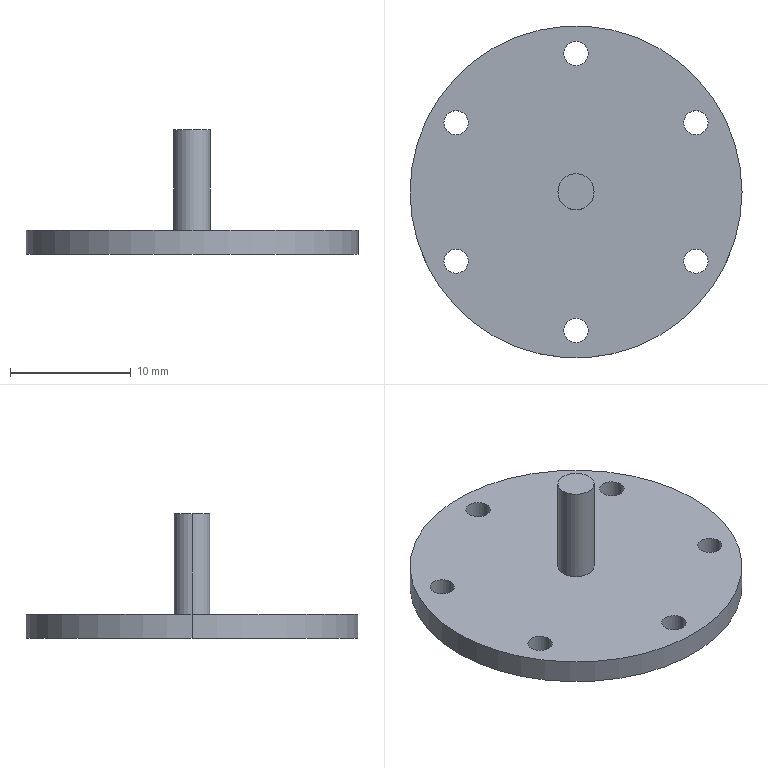Part | SolidWorks | features BaseBody 1 | 1 solid | 19 faces | box 27.511 x 27.511 x 10.35 mm | volume 1209 mm3 | cylinder 16 | plane 3 | commonest cylinder face diameters 2.021 x12 3 x2 27.511 x2
STEP:
#1=CARTESIAN_POINT('',(463.251,528.256,-2.));
#2=VERTEX_POINT('',#1);
#3=CARTESIAN_POINT('',(461.23,528.256,-2.));
#4=VERTEX_POINT('',#3);
#5=CARTESIAN_POINT('',(462.241,528.256,-2.));
#6=DIRECTION('',(0.,0.,-1.));
#7=DIRECTION('',(1.,0.,0.));
#8=AXIS2_PLACEMENT_3D('',#5,#6,#7);
#9=CIRCLE('',#8,1.011);
#10=EDGE_CURVE('',#2,#4,#9,.T.);
#11=ORIENTED_EDGE('',*,*,#10,.T.);
#12=CARTESIAN_POINT('',(461.23,528.256,0.));
#13=VERTEX_POINT('',#12);
#14=CARTESIAN_POINT('',(461.23,528.256,0.));
#15=DIRECTION('',(0.,0.,1.));
#16=VECTOR('',#15,1000.);
#17=LINE('',#14,#16);
#18=EDGE_CURVE('',#4,#13,#17,.T.);
#19=ORIENTED_EDGE('',*,*,#18,.T.);
#20=CARTESIAN_POINT('',(463.251,528.256,0.));
#21=VERTEX_POINT('',#20);
#22=CARTESIAN_POINT('',(462.241,528.256,0.));
#23=DIRECTION('',(0.,0.,-1.));
#24=DIRECTION('',(1.,0.,0.));
#25=AXIS2_PLACEMENT_3D('',#22,#23,#24);
#26=CIRCLE('',#25,1.011);
#27=EDGE_CURVE('',#21,#13,#26,.T.);
#28=ORIENTED_EDGE('',*,*,#27,.F.);
#29=CARTESIAN_POINT('',(463.251,528.256,0.));
#30=DIRECTION('',(0.,0.,1.));
#31=VECTOR('',#30,1000.);
#32=LINE('',#29,#31);
#33=EDGE_CURVE('',#2,#21,#32,.T.);
#34=ORIENTED_EDGE('',*,*,#33,.F.);
#35=EDGE_LOOP('',(#11,#19,#28,#34));
#36=FACE_OUTER_BOUND('',#35,.T.);
#37=CARTESIAN_POINT('',(462.241,528.256,0.));
#38=DIRECTION('',(0.,0.,1.));
#39=DIRECTION('',(1.,0.,0.));
#40=AXIS2_PLACEMENT_3D('',#37,#38,#39);
#41=CYLINDRICAL_SURFACE('',#40,1.011);
#42=ADVANCED_FACE('',(#36),#41,.F.);
#43=CARTESIAN_POINT('',(453.313,522.518,-2.));
#44=VERTEX_POINT('',#43);
#45=CARTESIAN_POINT('',(451.292,522.518,-2.));
#46=VERTEX_POINT('',#45);
#47=CARTESIAN_POINT('',(452.303,522.518,-2.));
#48=DIRECTION('',(0.,0.,-1.));
#49=DIRECTION('',(1.,0.,0.));
#50=AXIS2_PLACEMENT_3D('',#47,#48,#49);
#51=CIRCLE('',#50,1.011);
#52=EDGE_CURVE('',#44,#46,#51,.T.);
#53=ORIENTED_EDGE('',*,*,#52,.T.);
#54=CARTESIAN_POINT('',(451.292,522.518,0.));
#55=VERTEX_POINT('',#54);
#56=CARTESIAN_POINT('',(451.292,522.518,0.));
#57=DIRECTION('',(0.,0.,1.));
#58=VECTOR('',#57,1000.);
#59=LINE('',#56,#58);
#60=EDGE_CURVE('',#46,#55,#59,.T.);
#61=ORIENTED_EDGE('',*,*,#60,.T.);
#62=CARTESIAN_POINT('',(453.313,522.518,0.));
#63=VERTEX_POINT('',#62);
#64=CARTESIAN_POINT('',(452.303,522.518,0.));
#65=DIRECTION('',(0.,0.,-1.));
#66=DIRECTION('',(1.,0.,0.));
#67=AXIS2_PLACEMENT_3D('',#64,#65,#66);
#68=CIRCLE('',#67,1.011);
#69=EDGE_CURVE('',#63,#55,#68,.T.);
#70=ORIENTED_EDGE('',*,*,#69,.F.);
#71=CARTESIAN_POINT('',(453.313,522.518,0.));
#72=DIRECTION('',(0.,0.,1.));
#73=VECTOR('',#72,1000.);
#74=LINE('',#71,#73);
#75=EDGE_CURVE('',#44,#63,#74,.T.);
#76=ORIENTED_EDGE('',*,*,#75,.F.);
#77=EDGE_LOOP('',(#53,#61,#70,#76));
#78=FACE_OUTER_BOUND('',#77,.T.);
#79=CARTESIAN_POINT('',(452.303,522.518,0.));
#80=DIRECTION('',(0.,0.,1.));
#81=DIRECTION('',(1.,0.,0.));
#82=AXIS2_PLACEMENT_3D('',#79,#80,#81);
#83=CYLINDRICAL_SURFACE('',#82,1.011);
#84=ADVANCED_FACE('',(#78),#83,.F.);
#85=CARTESIAN_POINT('',(453.313,511.042,-2.));
#86=VERTEX_POINT('',#85);
#87=CARTESIAN_POINT('',(451.292,511.042,-2.));
#88=VERTEX_POINT('',#87);
#89=CARTESIAN_POINT('',(452.303,511.042,-2.));
#90=DIRECTION('',(0.,0.,-1.));
#91=DIRECTION('',(1.,0.,0.));
#92=AXIS2_PLACEMENT_3D('',#89,#90,#91);
#93=CIRCLE('',#92,1.011);
#94=EDGE_CURVE('',#86,#88,#93,.T.);
#95=ORIENTED_EDGE('',*,*,#94,.T.);
#96=CARTESIAN_POINT('',(451.292,511.042,0.));
#97=VERTEX_POINT('',#96);
#98=CARTESIAN_POINT('',(451.292,511.042,0.));
#99=DIRECTION('',(0.,0.,1.));
#100=VECTOR('',#99,1000.);
#101=LINE('',#98,#100);
#102=EDGE_CURVE('',#88,#97,#101,.T.);
#103=ORIENTED_EDGE('',*,*,#102,.T.);
#104=CARTESIAN_POINT('',(453.313,511.042,0.));
#105=VERTEX_POINT('',#104);
#106=CARTESIAN_POINT('',(452.303,511.042,0.));
#107=DIRECTION('',(0.,0.,-1.));
#108=DIRECTION('',(1.,0.,0.));
#109=AXIS2_PLACEMENT_3D('',#106,#107,#108);
#110=CIRCLE('',#109,1.011);
#111=EDGE_CURVE('',#105,#97,#110,.T.);
#112=ORIENTED_EDGE('',*,*,#111,.F.);
#113=CARTESIAN_POINT('',(453.313,511.042,0.));
#114=DIRECTION('',(0.,0.,1.));
#115=VECTOR('',#114,1000.);
#116=LINE('',#113,#115);
#117=EDGE_CURVE('',#86,#105,#116,.T.);
#118=ORIENTED_EDGE('',*,*,#117,.F.);
#119=EDGE_LOOP('',(#95,#103,#112,#118));
#120=FACE_OUTER_BOUND('',#119,.T.);
#121=CARTESIAN_POINT('',(452.303,511.042,0.));
#122=DIRECTION('',(0.,0.,1.));
#123=DIRECTION('',(1.,0.,0.));
#124=AXIS2_PLACEMENT_3D('',#121,#122,#123);
#125=CYLINDRICAL_SURFACE('',#124,1.011);
#126=ADVANCED_FACE('',(#120),#125,.F.);
#127=CARTESIAN_POINT('',(463.251,505.304,-2.));
#128=VERTEX_POINT('',#127);
#129=CARTESIAN_POINT('',(461.23,505.304,-2.));
#130=VERTEX_POINT('',#129);
#131=CARTESIAN_POINT('',(462.241,505.304,-2.));
#132=DIRECTION('',(0.,0.,-1.));
#133=DIRECTION('',(1.,0.,0.));
#134=AXIS2_PLACEMENT_3D('',#131,#132,#133);
#135=CIRCLE('',#134,1.011);
#136=EDGE_CURVE('',#128,#130,#135,.T.);
#137=ORIENTED_EDGE('',*,*,#136,.T.);
#138=CARTESIAN_POINT('',(461.23,505.304,0.));
#139=VERTEX_POINT('',#138);
#140=CARTESIAN_POINT('',(461.23,505.304,0.));
#141=DIRECTION('',(0.,0.,1.));
#142=VECTOR('',#141,1000.);
#143=LINE('',#140,#142);
#144=EDGE_CURVE('',#130,#139,#143,.T.);
#145=ORIENTED_EDGE('',*,*,#144,.T.);
#146=CARTESIAN_POINT('',(463.251,505.304,0.));
#147=VERTEX_POINT('',#146);
#148=CARTESIAN_POINT('',(462.241,505.304,0.));
#149=DIRECTION('',(0.,0.,-1.));
#150=DIRECTION('',(1.,0.,0.));
#151=AXIS2_PLACEMENT_3D('',#148,#149,#150);
#152=CIRCLE('',#151,1.011);
#153=EDGE_CURVE('',#147,#139,#152,.T.);
#154=ORIENTED_EDGE('',*,*,#153,.F.);
#155=CARTESIAN_POINT('',(463.251,505.304,0.));
#156=DIRECTION('',(0.,0.,1.));
#157=VECTOR('',#156,1000.);
#158=LINE('',#155,#157);
#159=EDGE_CURVE('',#128,#147,#158,.T.);
#160=ORIENTED_EDGE('',*,*,#159,.F.);
#161=EDGE_LOOP('',(#137,#145,#154,#160));
#162=FACE_OUTER_BOUND('',#161,.T.);
#163=CARTESIAN_POINT('',(462.241,505.304,0.));
#164=DIRECTION('',(0.,0.,1.));
#165=DIRECTION('',(1.,0.,0.));
#166=AXIS2_PLACEMENT_3D('',#163,#164,#165);
#167=CYLINDRICAL_SURFACE('',#166,1.011);
#168=ADVANCED_FACE('',(#162),#167,.F.);
#169=CARTESIAN_POINT('',(473.19,511.042,-2.));
#170=VERTEX_POINT('',#169);
#171=CARTESIAN_POINT('',(471.168,511.042,-2.));
#172=VERTEX_POINT('',#171);
#173=CARTESIAN_POINT('',(472.179,511.042,-2.));
#174=DIRECTION('',(0.,0.,-1.));
#175=DIRECTION('',(1.,0.,0.));
#176=AXIS2_PLACEMENT_3D('',#173,#174,#175);
#177=CIRCLE('',#176,1.011);
#178=EDGE_CURVE('',#170,#172,#177,.T.);
#179=ORIENTED_EDGE('',*,*,#178,.T.);
#180=CARTESIAN_POINT('',(471.168,511.042,0.));
#181=VERTEX_POINT('',#180);
#182=CARTESIAN_POINT('',(471.168,511.042,0.));
#183=DIRECTION('',(0.,0.,1.));
#184=VECTOR('',#183,1000.);
#185=LINE('',#182,#184);
#186=EDGE_CURVE('',#172,#181,#185,.T.);
#187=ORIENTED_EDGE('',*,*,#186,.T.);
#188=CARTESIAN_POINT('',(473.19,511.042,0.));
#189=VERTEX_POINT('',#188);
#190=CARTESIAN_POINT('',(472.179,511.042,0.));
#191=DIRECTION('',(0.,0.,-1.));
#192=DIRECTION('',(1.,0.,0.));
#193=AXIS2_PLACEMENT_3D('',#190,#191,#192);
#194=CIRCLE('',#193,1.011);
#195=EDGE_CURVE('',#189,#181,#194,.T.);
#196=ORIENTED_EDGE('',*,*,#195,.F.);
#197=CARTESIAN_POINT('',(473.19,511.042,0.));
#198=DIRECTION('',(0.,0.,1.));
#199=VECTOR('',#198,1000.);
#200=LINE('',#197,#199);
#201=EDGE_CURVE('',#170,#189,#200,.T.);
#202=ORIENTED_EDGE('',*,*,#201,.F.);
#203=EDGE_LOOP('',(#179,#187,#196,#202));
#204=FACE_OUTER_BOUND('',#203,.T.);
#205=CARTESIAN_POINT('',(472.179,511.042,0.));
#206=DIRECTION('',(0.,0.,1.));
#207=DIRECTION('',(1.,0.,0.));
#208=AXIS2_PLACEMENT_3D('',#205,#206,#207);
#209=CYLINDRICAL_SURFACE('',#208,1.011);
#210=ADVANCED_FACE('',(#204),#209,.F.);
#211=CARTESIAN_POINT('',(473.19,522.518,-2.));
#212=VERTEX_POINT('',#211);
#213=CARTESIAN_POINT('',(471.168,522.518,-2.));
#214=VERTEX_POINT('',#213);
#215=CARTESIAN_POINT('',(472.179,522.518,-2.));
#216=DIRECTION('',(0.,0.,-1.));
#217=DIRECTION('',(1.,0.,0.));
#218=AXIS2_PLACEMENT_3D('',#215,#216,#217);
#219=CIRCLE('',#218,1.011);
#220=EDGE_CURVE('',#212,#214,#219,.T.);
#221=ORIENTED_EDGE('',*,*,#220,.T.);
#222=CARTESIAN_POINT('',(471.168,522.518,0.));
#223=VERTEX_POINT('',#222);
#224=CARTESIAN_POINT('',(471.168,522.518,0.));
#225=DIRECTION('',(0.,0.,1.));
#226=VECTOR('',#225,1000.);
#227=LINE('',#224,#226);
#228=EDGE_CURVE('',#214,#223,#227,.T.);
#229=ORIENTED_EDGE('',*,*,#228,.T.);
#230=CARTESIAN_POINT('',(473.19,522.518,0.));
#231=VERTEX_POINT('',#230);
#232=CARTESIAN_POINT('',(472.179,522.518,0.));
#233=DIRECTION('',(0.,0.,-1.));
#234=DIRECTION('',(1.,0.,0.));
#235=AXIS2_PLACEMENT_3D('',#232,#233,#234);
#236=CIRCLE('',#235,1.011);
#237=EDGE_CURVE('',#231,#223,#236,.T.);
#238=ORIENTED_EDGE('',*,*,#237,.F.);
#239=CARTESIAN_POINT('',(473.19,522.518,0.));
#240=DIRECTION('',(0.,0.,1.));
#241=VECTOR('',#240,1000.);
#242=LINE('',#239,#241);
#243=EDGE_CURVE('',#212,#231,#242,.T.);
#244=ORIENTED_EDGE('',*,*,#243,.F.);
#245=EDGE_LOOP('',(#221,#229,#238,#244));
#246=FACE_OUTER_BOUND('',#245,.T.);
#247=CARTESIAN_POINT('',(472.179,522.518,0.));
#248=DIRECTION('',(0.,0.,1.));
#249=DIRECTION('',(1.,0.,0.));
#250=AXIS2_PLACEMENT_3D('',#247,#248,#249);
#251=CYLINDRICAL_SURFACE('',#250,1.011);
#252=ADVANCED_FACE('',(#246),#251,.F.);
#253=CARTESIAN_POINT('',(475.997,516.78,-2.));
#254=VERTEX_POINT('',#253);
#255=CARTESIAN_POINT('',(448.485,516.78,-2.));
#256=VERTEX_POINT('',#255);
#257=CARTESIAN_POINT('',(462.241,516.78,-2.));
#258=DIRECTION('',(0.,0.,1.));
#259=DIRECTION('',(1.,0.,0.));
#260=AXIS2_PLACEMENT_3D('',#257,#258,#259);
#261=CIRCLE('',#260,13.756);
#262=EDGE_CURVE('',#254,#256,#261,.T.);
#263=ORIENTED_EDGE('',*,*,#262,.T.);
#264=CARTESIAN_POINT('',(448.485,516.78,0.));
#265=VERTEX_POINT('',#264);
#266=CARTESIAN_POINT('',(448.485,516.78,0.));
#267=DIRECTION('',(0.,0.,1.));
#268=VECTOR('',#267,1000.);
#269=LINE('',#266,#268);
#270=EDGE_CURVE('',#256,#265,#269,.T.);
#271=ORIENTED_EDGE('',*,*,#270,.T.);
#272=CARTESIAN_POINT('',(475.997,516.78,0.));
#273=VERTEX_POINT('',#272);
#274=CARTESIAN_POINT('',(462.241,516.78,0.));
#275=DIRECTION('',(0.,0.,-1.));
#276=DIRECTION('',(1.,0.,0.));
#277=AXIS2_PLACEMENT_3D('',#274,#275,#276);
#278=CIRCLE('',#277,13.756);
#279=EDGE_CURVE('',#265,#273,#278,.T.);
#280=ORIENTED_EDGE('',*,*,#279,.T.);
#281=CARTESIAN_POINT('',(475.997,516.78,0.));
#282=DIRECTION('',(0.,0.,1.));
#283=VECTOR('',#282,1000.);
#284=LINE('',#281,#283);
#285=EDGE_CURVE('',#254,#273,#284,.T.);
#286=ORIENTED_EDGE('',*,*,#285,.F.);
#287=EDGE_LOOP('',(#263,#271,#280,#286));
#288=FACE_OUTER_BOUND('',#287,.T.);
#289=CARTESIAN_POINT('',(462.241,516.78,0.));
#290=DIRECTION('',(0.,0.,1.));
#291=DIRECTION('',(1.,0.,0.));
#292=AXIS2_PLACEMENT_3D('',#289,#290,#291);
#293=CYLINDRICAL_SURFACE('',#292,13.756);
#294=ADVANCED_FACE('',(#288),#293,.T.);
#295=CARTESIAN_POINT('',(460.741,516.78,8.35));
#296=VERTEX_POINT('',#295);
#297=CARTESIAN_POINT('',(463.741,516.78,8.35));
#298=VERTEX_POINT('',#297);
#299=CARTESIAN_POINT('',(462.241,516.78,8.35));
#300=DIRECTION('',(0.,0.,-1.));
#301=DIRECTION('',(-1.,0.,0.));
#302=AXIS2_PLACEMENT_3D('',#299,#300,#301);
#303=CIRCLE('',#302,1.5);
#304=EDGE_CURVE('',#296,#298,#303,.T.);
#305=ORIENTED_EDGE('',*,*,#304,.T.);
#306=CARTESIAN_POINT('',(463.741,516.78,0.));
#307=VERTEX_POINT('',#306);
#308=CARTESIAN_POINT('',(463.741,516.78,0.));
#309=DIRECTION('',(0.,0.,-1.));
#310=VECTOR('',#309,1000.);
#311=LINE('',#308,#310);
#312=EDGE_CURVE('',#298,#307,#311,.T.);
#313=ORIENTED_EDGE('',*,*,#312,.T.);
#314=CARTESIAN_POINT('',(460.741,516.78,0.));
#315=VERTEX_POINT('',#314);
#316=CARTESIAN_POINT('',(462.241,516.78,0.));
#317=DIRECTION('',(0.,0.,-1.));
#318=DIRECTION('',(-1.,0.,0.));
#319=AXIS2_PLACEMENT_3D('',#316,#317,#318);
#320=CIRCLE('',#319,1.5);
#321=EDGE_CURVE('',#315,#307,#320,.T.);
#322=ORIENTED_EDGE('',*,*,#321,.F.);
#323=CARTESIAN_POINT('',(460.741,516.78,0.));
#324=DIRECTION('',(0.,0.,-1.));
#325=VECTOR('',#324,1000.);
#326=LINE('',#323,#325);
#327=EDGE_CURVE('',#296,#315,#326,.T.);
#328=ORIENTED_EDGE('',*,*,#327,.F.);
#329=EDGE_LOOP('',(#305,#313,#322,#328));
#330=FACE_OUTER_BOUND('',#329,.T.);
#331=CARTESIAN_POINT('',(462.241,516.78,0.));
#332=DIRECTION('',(0.,0.,-1.));
#333=DIRECTION('',(-1.,0.,0.));
#334=AXIS2_PLACEMENT_3D('',#331,#332,#333);
#335=CYLINDRICAL_SURFACE('',#334,1.5);
#336=ADVANCED_FACE('',(#330),#335,.T.);
#337=ORIENTED_EDGE('',*,*,#10,.F.);
#338=CARTESIAN_POINT('',(462.241,528.256,-2.));
#339=DIRECTION('',(0.,0.,-1.));
#340=DIRECTION('',(1.,0.,0.));
#341=AXIS2_PLACEMENT_3D('',#338,#339,#340);
#342=CIRCLE('',#341,1.011);
#343=EDGE_CURVE('',#4,#2,#342,.T.);
#344=ORIENTED_EDGE('',*,*,#343,.F.);
#345=EDGE_LOOP('',(#337,#344));
#346=FACE_BOUND('',#345,.T.);
#347=ORIENTED_EDGE('',*,*,#52,.F.);
#348=CARTESIAN_POINT('',(452.303,522.518,-2.));
#349=DIRECTION('',(0.,0.,-1.));
#350=DIRECTION('',(1.,0.,0.));
#351=AXIS2_PLACEMENT_3D('',#348,#349,#350);
#352=CIRCLE('',#351,1.011);
#353=EDGE_CURVE('',#46,#44,#352,.T.);
#354=ORIENTED_EDGE('',*,*,#353,.F.);
#355=EDGE_LOOP('',(#347,#354));
#356=FACE_BOUND('',#355,.T.);
#357=ORIENTED_EDGE('',*,*,#94,.F.);
#358=CARTESIAN_POINT('',(452.303,511.042,-2.));
#359=DIRECTION('',(0.,0.,-1.));
#360=DIRECTION('',(1.,0.,0.));
#361=AXIS2_PLACEMENT_3D('',#358,#359,#360);
#362=CIRCLE('',#361,1.011);
#363=EDGE_CURVE('',#88,#86,#362,.T.);
#364=ORIENTED_EDGE('',*,*,#363,.F.);
#365=EDGE_LOOP('',(#357,#364));
#366=FACE_BOUND('',#365,.T.);
#367=ORIENTED_EDGE('',*,*,#136,.F.);
#368=CARTESIAN_POINT('',(462.241,505.304,-2.));
#369=DIRECTION('',(0.,0.,-1.));
#370=DIRECTION('',(1.,0.,0.));
#371=AXIS2_PLACEMENT_3D('',#368,#369,#370);
#372=CIRCLE('',#371,1.011);
#373=EDGE_CURVE('',#130,#128,#372,.T.);
#374=ORIENTED_EDGE('',*,*,#373,.F.);
#375=EDGE_LOOP('',(#367,#374));
#376=FACE_BOUND('',#375,.T.);
#377=ORIENTED_EDGE('',*,*,#178,.F.);
#378=CARTESIAN_POINT('',(472.179,511.042,-2.));
#379=DIRECTION('',(0.,0.,-1.));
#380=DIRECTION('',(1.,0.,0.));
#381=AXIS2_PLACEMENT_3D('',#378,#379,#380);
#382=CIRCLE('',#381,1.011);
#383=EDGE_CURVE('',#172,#170,#382,.T.);
#384=ORIENTED_EDGE('',*,*,#383,.F.);
#385=EDGE_LOOP('',(#377,#384));
#386=FACE_BOUND('',#385,.T.);
#387=ORIENTED_EDGE('',*,*,#220,.F.);
#388=CARTESIAN_POINT('',(472.179,522.518,-2.));
#389=DIRECTION('',(0.,0.,-1.));
#390=DIRECTION('',(1.,0.,0.));
#391=AXIS2_PLACEMENT_3D('',#388,#389,#390);
#392=CIRCLE('',#391,1.011);
#393=EDGE_CURVE('',#214,#212,#392,.T.);
#394=ORIENTED_EDGE('',*,*,#393,.F.);
#395=EDGE_LOOP('',(#387,#394));
#396=FACE_BOUND('',#395,.T.);
#397=ORIENTED_EDGE('',*,*,#262,.F.);
#398=CARTESIAN_POINT('',(462.241,516.78,-2.));
#399=DIRECTION('',(0.,0.,1.));
#400=DIRECTION('',(1.,0.,0.));
#401=AXIS2_PLACEMENT_3D('',#398,#399,#400);
#402=CIRCLE('',#401,13.756);
#403=EDGE_CURVE('',#256,#254,#402,.T.);
#404=ORIENTED_EDGE('',*,*,#403,.F.);
#405=EDGE_LOOP('',(#397,#404));
#406=FACE_OUTER_BOUND('',#405,.T.);
#407=CARTESIAN_POINT('',(462.241,516.78,-2.));
#408=DIRECTION('',(0.,0.,1.));
#409=DIRECTION('',(1.,0.,0.));
#410=AXIS2_PLACEMENT_3D('',#407,#408,#409);
#411=PLANE('',#410);
#412=ADVANCED_FACE('',(#346,#356,#366,#376,#386,#396,#406),#411,.F.);
#413=ORIENTED_EDGE('',*,*,#18,.F.);
#414=ORIENTED_EDGE('',*,*,#343,.T.);
#415=ORIENTED_EDGE('',*,*,#33,.T.);
#416=CARTESIAN_POINT('',(462.241,528.256,0.));
#417=DIRECTION('',(0.,0.,-1.));
#418=DIRECTION('',(1.,0.,0.));
#419=AXIS2_PLACEMENT_3D('',#416,#417,#418);
#420=CIRCLE('',#419,1.011);
#421=EDGE_CURVE('',#13,#21,#420,.T.);
#422=ORIENTED_EDGE('',*,*,#421,.F.);
#423=EDGE_LOOP('',(#413,#414,#415,#422));
#424=FACE_OUTER_BOUND('',#423,.T.);
#425=CARTESIAN_POINT('',(462.241,528.256,0.));
#426=DIRECTION('',(0.,0.,1.));
#427=DIRECTION('',(1.,0.,0.));
#428=AXIS2_PLACEMENT_3D('',#425,#426,#427);
#429=CYLINDRICAL_SURFACE('',#428,1.011);
#430=ADVANCED_FACE('',(#424),#429,.F.);
#431=ORIENTED_EDGE('',*,*,#60,.F.);
#432=ORIENTED_EDGE('',*,*,#353,.T.);
#433=ORIENTED_EDGE('',*,*,#75,.T.);
#434=CARTESIAN_POINT('',(452.303,522.518,0.));
#435=DIRECTION('',(0.,0.,-1.));
#436=DIRECTION('',(1.,0.,0.));
#437=AXIS2_PLACEMENT_3D('',#434,#435,#436);
#438=CIRCLE('',#437,1.011);
#439=EDGE_CURVE('',#55,#63,#438,.T.);
#440=ORIENTED_EDGE('',*,*,#439,.F.);
#441=EDGE_LOOP('',(#431,#432,#433,#440));
#442=FACE_OUTER_BOUND('',#441,.T.);
#443=CARTESIAN_POINT('',(452.303,522.518,0.));
#444=DIRECTION('',(0.,0.,1.));
#445=DIRECTION('',(1.,0.,0.));
#446=AXIS2_PLACEMENT_3D('',#443,#444,#445);
#447=CYLINDRICAL_SURFACE('',#446,1.011);
#448=ADVANCED_FACE('',(#442),#447,.F.);
#449=ORIENTED_EDGE('',*,*,#102,.F.);
#450=ORIENTED_EDGE('',*,*,#363,.T.);
#451=ORIENTED_EDGE('',*,*,#117,.T.);
#452=CARTESIAN_POINT('',(452.303,511.042,0.));
#453=DIRECTION('',(0.,0.,-1.));
#454=DIRECTION('',(1.,0.,0.));
#455=AXIS2_PLACEMENT_3D('',#452,#453,#454);
#456=CIRCLE('',#455,1.011);
#457=EDGE_CURVE('',#97,#105,#456,.T.);
#458=ORIENTED_EDGE('',*,*,#457,.F.);
#459=EDGE_LOOP('',(#449,#450,#451,#458));
#460=FACE_OUTER_BOUND('',#459,.T.);
#461=CARTESIAN_POINT('',(452.303,511.042,0.));
#462=DIRECTION('',(0.,0.,1.));
#463=DIRECTION('',(1.,0.,0.));
#464=AXIS2_PLACEMENT_3D('',#461,#462,#463);
#465=CYLINDRICAL_SURFACE('',#464,1.011);
#466=ADVANCED_FACE('',(#460),#465,.F.);
#467=ORIENTED_EDGE('',*,*,#144,.F.);
#468=ORIENTED_EDGE('',*,*,#373,.T.);
#469=ORIENTED_EDGE('',*,*,#159,.T.);
#470=CARTESIAN_POINT('',(462.241,505.304,0.));
#471=DIRECTION('',(0.,0.,-1.));
#472=DIRECTION('',(1.,0.,0.));
#473=AXIS2_PLACEMENT_3D('',#470,#471,#472);
#474=CIRCLE('',#473,1.011);
#475=EDGE_CURVE('',#139,#147,#474,.T.);
#476=ORIENTED_EDGE('',*,*,#475,.F.);
#477=EDGE_LOOP('',(#467,#468,#469,#476));
#478=FACE_OUTER_BOUND('',#477,.T.);
#479=CARTESIAN_POINT('',(462.241,505.304,0.));
#480=DIRECTION('',(0.,0.,1.));
#481=DIRECTION('',(1.,0.,0.));
#482=AXIS2_PLACEMENT_3D('',#479,#480,#481);
#483=CYLINDRICAL_SURFACE('',#482,1.011);
#484=ADVANCED_FACE('',(#478),#483,.F.);
#485=ORIENTED_EDGE('',*,*,#186,.F.);
#486=ORIENTED_EDGE('',*,*,#383,.T.);
#487=ORIENTED_EDGE('',*,*,#201,.T.);
#488=CARTESIAN_POINT('',(472.179,511.042,0.));
#489=DIRECTION('',(0.,0.,-1.));
#490=DIRECTION('',(1.,0.,0.));
#491=AXIS2_PLACEMENT_3D('',#488,#489,#490);
#492=CIRCLE('',#491,1.011);
#493=EDGE_CURVE('',#181,#189,#492,.T.);
#494=ORIENTED_EDGE('',*,*,#493,.F.);
#495=EDGE_LOOP('',(#485,#486,#487,#494));
#496=FACE_OUTER_BOUND('',#495,.T.);
#497=CARTESIAN_POINT('',(472.179,511.042,0.));
#498=DIRECTION('',(0.,0.,1.));
#499=DIRECTION('',(1.,0.,0.));
#500=AXIS2_PLACEMENT_3D('',#497,#498,#499);
#501=CYLINDRICAL_SURFACE('',#500,1.011);
#502=ADVANCED_FACE('',(#496),#501,.F.);
#503=ORIENTED_EDGE('',*,*,#228,.F.);
#504=ORIENTED_EDGE('',*,*,#393,.T.);
#505=ORIENTED_EDGE('',*,*,#243,.T.);
#506=CARTESIAN_POINT('',(472.179,522.518,0.));
#507=DIRECTION('',(0.,0.,-1.));
#508=DIRECTION('',(1.,0.,0.));
#509=AXIS2_PLACEMENT_3D('',#506,#507,#508);
#510=CIRCLE('',#509,1.011);
#511=EDGE_CURVE('',#223,#231,#510,.T.);
#512=ORIENTED_EDGE('',*,*,#511,.F.);
#513=EDGE_LOOP('',(#503,#504,#505,#512));
#514=FACE_OUTER_BOUND('',#513,.T.);
#515=CARTESIAN_POINT('',(472.179,522.518,0.));
#516=DIRECTION('',(0.,0.,1.));
#517=DIRECTION('',(1.,0.,0.));
#518=AXIS2_PLACEMENT_3D('',#515,#516,#517);
#519=CYLINDRICAL_SURFACE('',#518,1.011);
#520=ADVANCED_FACE('',(#514),#519,.F.);
#521=ORIENTED_EDGE('',*,*,#270,.F.);
#522=ORIENTED_EDGE('',*,*,#403,.T.);
#523=ORIENTED_EDGE('',*,*,#285,.T.);
#524=CARTESIAN_POINT('',(462.241,516.78,0.));
#525=DIRECTION('',(0.,0.,-1.));
#526=DIRECTION('',(1.,0.,0.));
#527=AXIS2_PLACEMENT_3D('',#524,#525,#526);
#528=CIRCLE('',#527,13.756);
#529=EDGE_CURVE('',#273,#265,#528,.T.);
#530=ORIENTED_EDGE('',*,*,#529,.T.);
#531=EDGE_LOOP('',(#521,#522,#523,#530));
#532=FACE_OUTER_BOUND('',#531,.T.);
#533=CARTESIAN_POINT('',(462.241,516.78,0.));
#534=DIRECTION('',(0.,0.,1.));
#535=DIRECTION('',(1.,0.,0.));
#536=AXIS2_PLACEMENT_3D('',#533,#534,#535);
#537=CYLINDRICAL_SURFACE('',#536,13.756);
#538=ADVANCED_FACE('',(#532),#537,.T.);
#539=ORIENTED_EDGE('',*,*,#27,.T.);
#540=ORIENTED_EDGE('',*,*,#421,.T.);
#541=EDGE_LOOP('',(#539,#540));
#542=FACE_BOUND('',#541,.T.);
#543=ORIENTED_EDGE('',*,*,#69,.T.);
#544=ORIENTED_EDGE('',*,*,#439,.T.);
#545=EDGE_LOOP('',(#543,#544));
#546=FACE_BOUND('',#545,.T.);
#547=ORIENTED_EDGE('',*,*,#111,.T.);
#548=ORIENTED_EDGE('',*,*,#457,.T.);
#549=EDGE_LOOP('',(#547,#548));
#550=FACE_BOUND('',#549,.T.);
#551=ORIENTED_EDGE('',*,*,#153,.T.);
#552=ORIENTED_EDGE('',*,*,#475,.T.);
#553=EDGE_LOOP('',(#551,#552));
#554=FACE_BOUND('',#553,.T.);
#555=ORIENTED_EDGE('',*,*,#195,.T.);
#556=ORIENTED_EDGE('',*,*,#493,.T.);
#557=EDGE_LOOP('',(#555,#556));
#558=FACE_BOUND('',#557,.T.);
#559=ORIENTED_EDGE('',*,*,#237,.T.);
#560=ORIENTED_EDGE('',*,*,#511,.T.);
#561=EDGE_LOOP('',(#559,#560));
#562=FACE_BOUND('',#561,.T.);
#563=ORIENTED_EDGE('',*,*,#321,.T.);
#564=CARTESIAN_POINT('',(462.241,516.78,0.));
#565=DIRECTION('',(0.,0.,-1.));
#566=DIRECTION('',(-1.,0.,0.));
#567=AXIS2_PLACEMENT_3D('',#564,#565,#566);
#568=CIRCLE('',#567,1.5);
#569=EDGE_CURVE('',#307,#315,#568,.T.);
#570=ORIENTED_EDGE('',*,*,#569,.T.);
#571=EDGE_LOOP('',(#563,#570));
#572=FACE_BOUND('',#571,.T.);
#573=ORIENTED_EDGE('',*,*,#529,.F.);
#574=ORIENTED_EDGE('',*,*,#279,.F.);
#575=EDGE_LOOP('',(#573,#574));
#576=FACE_OUTER_BOUND('',#575,.T.);
#577=CARTESIAN_POINT('',(462.241,516.78,0.));
#578=DIRECTION('',(0.,0.,1.));
#579=DIRECTION('',(1.,0.,0.));
#580=AXIS2_PLACEMENT_3D('',#577,#578,#579);
#581=PLANE('',#580);
#582=ADVANCED_FACE('',(#542,#546,#550,#554,#558,#562,#572,#576),#581,.T.);
#583=ORIENTED_EDGE('',*,*,#312,.F.);
#584=CARTESIAN_POINT('',(462.241,516.78,8.35));
#585=DIRECTION('',(0.,0.,-1.));
#586=DIRECTION('',(-1.,0.,0.));
#587=AXIS2_PLACEMENT_3D('',#584,#585,#586);
#588=CIRCLE('',#587,1.5);
#589=EDGE_CURVE('',#298,#296,#588,.T.);
#590=ORIENTED_EDGE('',*,*,#589,.T.);
#591=ORIENTED_EDGE('',*,*,#327,.T.);
#592=ORIENTED_EDGE('',*,*,#569,.F.);
#593=EDGE_LOOP('',(#583,#590,#591,#592));
#594=FACE_OUTER_BOUND('',#593,.T.);
#595=CARTESIAN_POINT('',(462.241,516.78,0.));
#596=DIRECTION('',(0.,0.,-1.));
#597=DIRECTION('',(-1.,0.,0.));
#598=AXIS2_PLACEMENT_3D('',#595,#596,#597);
#599=CYLINDRICAL_SURFACE('',#598,1.5);
#600=ADVANCED_FACE('',(#594),#599,.T.);
#601=ORIENTED_EDGE('',*,*,#304,.F.);
#602=ORIENTED_EDGE('',*,*,#589,.F.);
#603=EDGE_LOOP('',(#601,#602));
#604=FACE_OUTER_BOUND('',#603,.T.);
#605=CARTESIAN_POINT('',(462.241,516.78,8.35));
#606=DIRECTION('',(0.,0.,-1.));
#607=DIRECTION('',(-1.,0.,0.));
#608=AXIS2_PLACEMENT_3D('',#605,#606,#607);
#609=PLANE('',#608);
#610=ADVANCED_FACE('',(#604),#609,.F.);
#611=CLOSED_SHELL('',(#42,#84,#126,#168,#210,#252,#294,#336,#412,#430,#448,#466,#484,#502,#520,#538,#582,#600,#610));
#612=MANIFOLD_SOLID_BREP('',#611);
#613=CARTESIAN_POINT('',(0.,0.,0.));
#614=DIRECTION('',(0.,0.,1.));
#615=DIRECTION('',(1.,0.,0.));
#616=AXIS2_PLACEMENT_3D('',#613,#614,#615);
#617=(LENGTH_UNIT()NAMED_UNIT(*)SI_UNIT(.MILLI.,.METRE.));
#618=UNCERTAINTY_MEASURE_WITH_UNIT(LENGTH_MEASURE(0.00001),#617,'','');
#619=(NAMED_UNIT(*)PLANE_ANGLE_UNIT()SI_UNIT($,.RADIAN.));
#620=(NAMED_UNIT(*)SI_UNIT($,.STERADIAN.)SOLID_ANGLE_UNIT());
#621=(GEOMETRIC_REPRESENTATION_CONTEXT(3)GLOBAL_UNCERTAINTY_ASSIGNED_CONTEXT((#618))GLOBAL_UNIT_ASSIGNED_CONTEXT((#617,#619,#620))REPRESENTATION_CONTEXT('',''));
#622=ADVANCED_BREP_SHAPE_REPRESENTATION('',(#612,#616),#621);